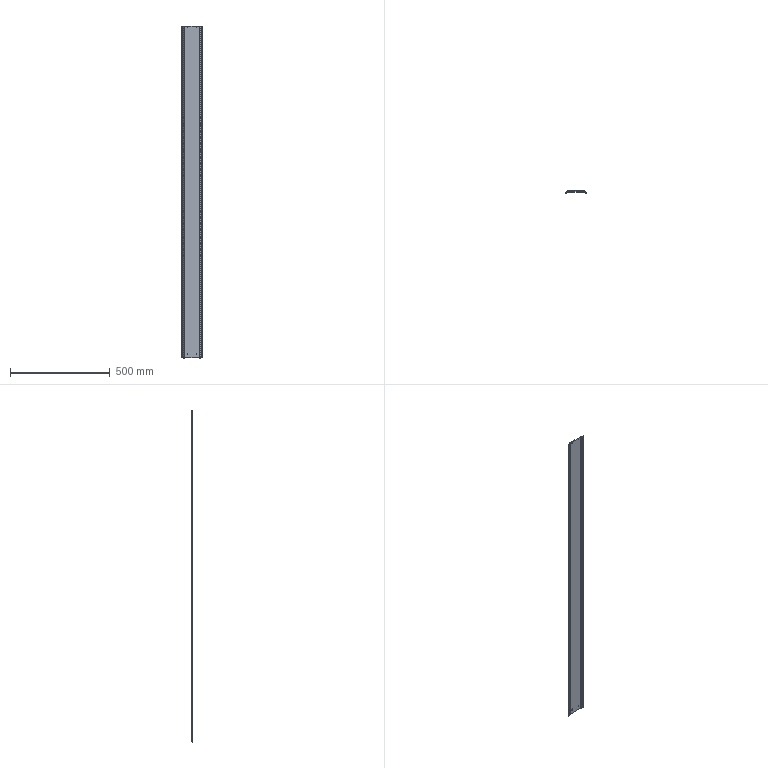Part | SolidWorks | features BaseBody 1 | 1 solid | 82 faces | box 109 x 8.5 x 1667 mm | volume 552829 mm3 | cylinder 40 | plane 22 | cone 20 | commonest cylinder face diameters 3.3 x12 3.4 x8 2 x7 3.2 x6 5.2 x5 0.399 x2